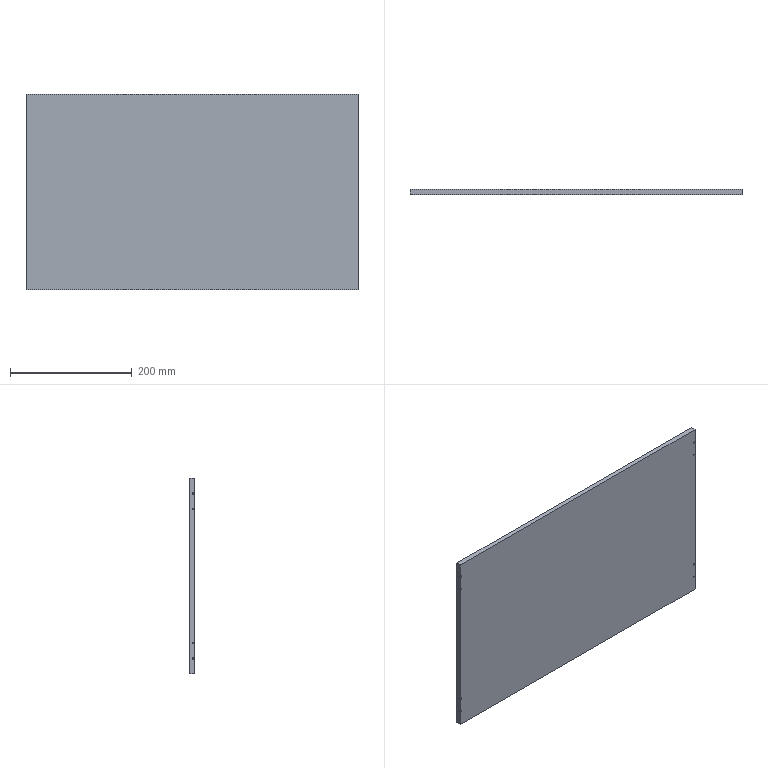Part | SolidWorks | features BaseBody 1 | 1 solid | 88 faces | box 545 x 7.9 x 320.7 mm | volume 1351854 mm3 | plane 72 | cylinder 16 | commonest cylinder face diameters 3 x16